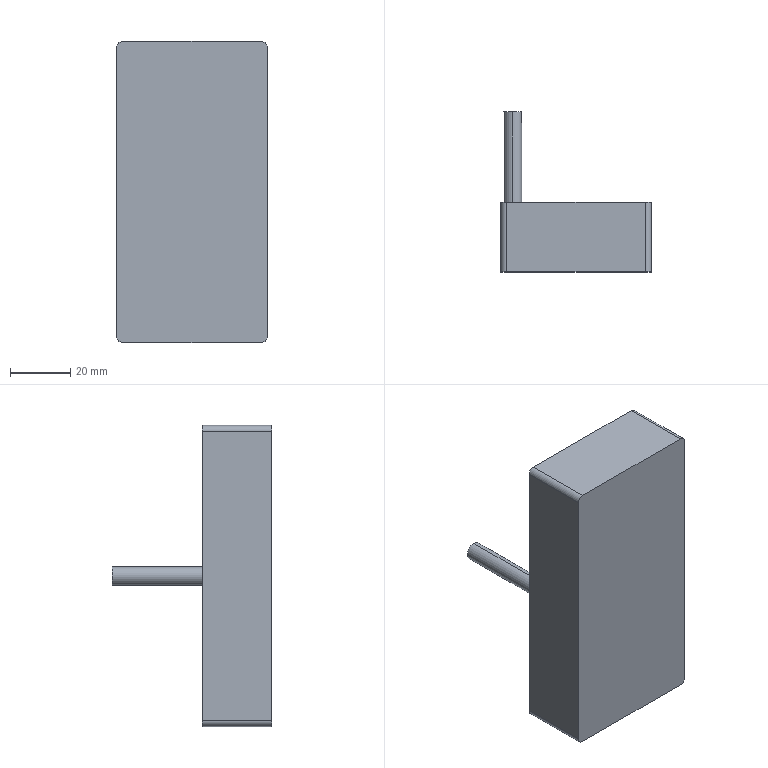Part | SolidWorks | features BaseBody 1 | 1 solid | 45 faces | box 50 x 53.1 x 100 mm | volume 115973 mm3 | cylinder 22 | cone 16 | plane 7 | commonest cylinder face diameters 3.3 x16 4 x4 6 x2
STEP:
#1=CARTESIAN_POINT('',(15.,19.1,86.85));
#2=VERTEX_POINT('',#1);
#3=CARTESIAN_POINT('',(15.,19.1,90.15));
#4=VERTEX_POINT('',#3);
#5=CARTESIAN_POINT('',(15.,19.1,88.5));
#6=DIRECTION('',(0.,1.,0.));
#7=DIRECTION('',(0.,0.,1.));
#8=AXIS2_PLACEMENT_3D('',#5,#6,#7);
#9=CIRCLE('',#8,1.65);
#10=EDGE_CURVE('',#2,#4,#9,.T.);
#11=ORIENTED_EDGE('',*,*,#10,.F.);
#12=CARTESIAN_POINT('',(15.,23.1,86.85));
#13=VERTEX_POINT('',#12);
#14=CARTESIAN_POINT('',(15.,23.1,86.85));
#15=DIRECTION('',(0.,1.,0.));
#16=VECTOR('',#15,1000.);
#17=LINE('',#14,#16);
#18=EDGE_CURVE('',#2,#13,#17,.T.);
#19=ORIENTED_EDGE('',*,*,#18,.T.);
#20=CARTESIAN_POINT('',(15.,23.1,90.15));
#21=VERTEX_POINT('',#20);
#22=CARTESIAN_POINT('',(15.,23.1,88.5));
#23=DIRECTION('',(0.,1.,0.));
#24=DIRECTION('',(0.,0.,1.));
#25=AXIS2_PLACEMENT_3D('',#22,#23,#24);
#26=CIRCLE('',#25,1.65);
#27=EDGE_CURVE('',#13,#21,#26,.T.);
#28=ORIENTED_EDGE('',*,*,#27,.T.);
#29=CARTESIAN_POINT('',(15.,23.1,90.15));
#30=DIRECTION('',(0.,1.,0.));
#31=VECTOR('',#30,1000.);
#32=LINE('',#29,#31);
#33=EDGE_CURVE('',#4,#21,#32,.T.);
#34=ORIENTED_EDGE('',*,*,#33,.F.);
#35=EDGE_LOOP('',(#11,#19,#28,#34));
#36=FACE_OUTER_BOUND('',#35,.T.);
#37=CARTESIAN_POINT('',(15.,23.1,88.5));
#38=DIRECTION('',(0.,1.,0.));
#39=DIRECTION('',(0.,0.,1.));
#40=AXIS2_PLACEMENT_3D('',#37,#38,#39);
#41=CYLINDRICAL_SURFACE('',#40,1.65);
#42=ADVANCED_FACE('',(#36),#41,.F.);
#43=CARTESIAN_POINT('',(15.,19.1,62.85));
#44=VERTEX_POINT('',#43);
#45=CARTESIAN_POINT('',(15.,19.1,66.15));
#46=VERTEX_POINT('',#45);
#47=CARTESIAN_POINT('',(15.,19.1,64.5));
#48=DIRECTION('',(0.,1.,0.));
#49=DIRECTION('',(0.,0.,1.));
#50=AXIS2_PLACEMENT_3D('',#47,#48,#49);
#51=CIRCLE('',#50,1.65);
#52=EDGE_CURVE('',#44,#46,#51,.T.);
#53=ORIENTED_EDGE('',*,*,#52,.F.);
#54=CARTESIAN_POINT('',(15.,23.1,62.85));
#55=VERTEX_POINT('',#54);
#56=CARTESIAN_POINT('',(15.,23.1,62.85));
#57=DIRECTION('',(0.,1.,0.));
#58=VECTOR('',#57,1000.);
#59=LINE('',#56,#58);
#60=EDGE_CURVE('',#44,#55,#59,.T.);
#61=ORIENTED_EDGE('',*,*,#60,.T.);
#62=CARTESIAN_POINT('',(15.,23.1,66.15));
#63=VERTEX_POINT('',#62);
#64=CARTESIAN_POINT('',(15.,23.1,64.5));
#65=DIRECTION('',(0.,1.,0.));
#66=DIRECTION('',(0.,0.,1.));
#67=AXIS2_PLACEMENT_3D('',#64,#65,#66);
#68=CIRCLE('',#67,1.65);
#69=EDGE_CURVE('',#55,#63,#68,.T.);
#70=ORIENTED_EDGE('',*,*,#69,.T.);
#71=CARTESIAN_POINT('',(15.,23.1,66.15));
#72=DIRECTION('',(0.,1.,0.));
#73=VECTOR('',#72,1000.);
#74=LINE('',#71,#73);
#75=EDGE_CURVE('',#46,#63,#74,.T.);
#76=ORIENTED_EDGE('',*,*,#75,.F.);
#77=EDGE_LOOP('',(#53,#61,#70,#76));
#78=FACE_OUTER_BOUND('',#77,.T.);
#79=CARTESIAN_POINT('',(15.,23.1,64.5));
#80=DIRECTION('',(0.,1.,0.));
#81=DIRECTION('',(0.,0.,1.));
#82=AXIS2_PLACEMENT_3D('',#79,#80,#81);
#83=CYLINDRICAL_SURFACE('',#82,1.65);
#84=ADVANCED_FACE('',(#78),#83,.F.);
#85=CARTESIAN_POINT('',(35.,19.1,86.85));
#86=VERTEX_POINT('',#85);
#87=CARTESIAN_POINT('',(35.,19.1,90.15));
#88=VERTEX_POINT('',#87);
#89=CARTESIAN_POINT('',(35.,19.1,88.5));
#90=DIRECTION('',(0.,1.,0.));
#91=DIRECTION('',(0.,0.,1.));
#92=AXIS2_PLACEMENT_3D('',#89,#90,#91);
#93=CIRCLE('',#92,1.65);
#94=EDGE_CURVE('',#86,#88,#93,.T.);
#95=ORIENTED_EDGE('',*,*,#94,.F.);
#96=CARTESIAN_POINT('',(35.,23.1,86.85));
#97=VERTEX_POINT('',#96);
#98=CARTESIAN_POINT('',(35.,23.1,86.85));
#99=DIRECTION('',(0.,1.,0.));
#100=VECTOR('',#99,1000.);
#101=LINE('',#98,#100);
#102=EDGE_CURVE('',#86,#97,#101,.T.);
#103=ORIENTED_EDGE('',*,*,#102,.T.);
#104=CARTESIAN_POINT('',(35.,23.1,90.15));
#105=VERTEX_POINT('',#104);
#106=CARTESIAN_POINT('',(35.,23.1,88.5));
#107=DIRECTION('',(0.,1.,0.));
#108=DIRECTION('',(0.,0.,1.));
#109=AXIS2_PLACEMENT_3D('',#106,#107,#108);
#110=CIRCLE('',#109,1.65);
#111=EDGE_CURVE('',#97,#105,#110,.T.);
#112=ORIENTED_EDGE('',*,*,#111,.T.);
#113=CARTESIAN_POINT('',(35.,23.1,90.15));
#114=DIRECTION('',(0.,1.,0.));
#115=VECTOR('',#114,1000.);
#116=LINE('',#113,#115);
#117=EDGE_CURVE('',#88,#105,#116,.T.);
#118=ORIENTED_EDGE('',*,*,#117,.F.);
#119=EDGE_LOOP('',(#95,#103,#112,#118));
#120=FACE_OUTER_BOUND('',#119,.T.);
#121=CARTESIAN_POINT('',(35.,23.1,88.5));
#122=DIRECTION('',(0.,1.,0.));
#123=DIRECTION('',(0.,0.,1.));
#124=AXIS2_PLACEMENT_3D('',#121,#122,#123);
#125=CYLINDRICAL_SURFACE('',#124,1.65);
#126=ADVANCED_FACE('',(#120),#125,.F.);
#127=CARTESIAN_POINT('',(35.,19.1,62.85));
#128=VERTEX_POINT('',#127);
#129=CARTESIAN_POINT('',(35.,19.1,66.15));
#130=VERTEX_POINT('',#129);
#131=CARTESIAN_POINT('',(35.,19.1,64.5));
#132=DIRECTION('',(0.,1.,0.));
#133=DIRECTION('',(0.,0.,1.));
#134=AXIS2_PLACEMENT_3D('',#131,#132,#133);
#135=CIRCLE('',#134,1.65);
#136=EDGE_CURVE('',#128,#130,#135,.T.);
#137=ORIENTED_EDGE('',*,*,#136,.F.);
#138=CARTESIAN_POINT('',(35.,23.1,62.85));
#139=VERTEX_POINT('',#138);
#140=CARTESIAN_POINT('',(35.,23.1,62.85));
#141=DIRECTION('',(0.,1.,0.));
#142=VECTOR('',#141,1000.);
#143=LINE('',#140,#142);
#144=EDGE_CURVE('',#128,#139,#143,.T.);
#145=ORIENTED_EDGE('',*,*,#144,.T.);
#146=CARTESIAN_POINT('',(35.,23.1,66.15));
#147=VERTEX_POINT('',#146);
#148=CARTESIAN_POINT('',(35.,23.1,64.5));
#149=DIRECTION('',(0.,1.,0.));
#150=DIRECTION('',(0.,0.,1.));
#151=AXIS2_PLACEMENT_3D('',#148,#149,#150);
#152=CIRCLE('',#151,1.65);
#153=EDGE_CURVE('',#139,#147,#152,.T.);
#154=ORIENTED_EDGE('',*,*,#153,.T.);
#155=CARTESIAN_POINT('',(35.,23.1,66.15));
#156=DIRECTION('',(0.,1.,0.));
#157=VECTOR('',#156,1000.);
#158=LINE('',#155,#157);
#159=EDGE_CURVE('',#130,#147,#158,.T.);
#160=ORIENTED_EDGE('',*,*,#159,.F.);
#161=EDGE_LOOP('',(#137,#145,#154,#160));
#162=FACE_OUTER_BOUND('',#161,.T.);
#163=CARTESIAN_POINT('',(35.,23.1,64.5));
#164=DIRECTION('',(0.,1.,0.));
#165=DIRECTION('',(0.,0.,1.));
#166=AXIS2_PLACEMENT_3D('',#163,#164,#165);
#167=CYLINDRICAL_SURFACE('',#166,1.65);
#168=ADVANCED_FACE('',(#162),#167,.F.);
#169=CARTESIAN_POINT('',(15.,19.1,14.85));
#170=VERTEX_POINT('',#169);
#171=CARTESIAN_POINT('',(15.,19.1,18.15));
#172=VERTEX_POINT('',#171);
#173=CARTESIAN_POINT('',(15.,19.1,16.5));
#174=DIRECTION('',(0.,1.,0.));
#175=DIRECTION('',(0.,0.,1.));
#176=AXIS2_PLACEMENT_3D('',#173,#174,#175);
#177=CIRCLE('',#176,1.65);
#178=EDGE_CURVE('',#170,#172,#177,.T.);
#179=ORIENTED_EDGE('',*,*,#178,.F.);
#180=CARTESIAN_POINT('',(15.,23.1,14.85));
#181=VERTEX_POINT('',#180);
#182=CARTESIAN_POINT('',(15.,23.1,14.85));
#183=DIRECTION('',(0.,1.,0.));
#184=VECTOR('',#183,1000.);
#185=LINE('',#182,#184);
#186=EDGE_CURVE('',#170,#181,#185,.T.);
#187=ORIENTED_EDGE('',*,*,#186,.T.);
#188=CARTESIAN_POINT('',(15.,23.1,18.15));
#189=VERTEX_POINT('',#188);
#190=CARTESIAN_POINT('',(15.,23.1,16.5));
#191=DIRECTION('',(0.,1.,0.));
#192=DIRECTION('',(0.,0.,1.));
#193=AXIS2_PLACEMENT_3D('',#190,#191,#192);
#194=CIRCLE('',#193,1.65);
#195=EDGE_CURVE('',#181,#189,#194,.T.);
#196=ORIENTED_EDGE('',*,*,#195,.T.);
#197=CARTESIAN_POINT('',(15.,23.1,18.15));
#198=DIRECTION('',(0.,1.,0.));
#199=VECTOR('',#198,1000.);
#200=LINE('',#197,#199);
#201=EDGE_CURVE('',#172,#189,#200,.T.);
#202=ORIENTED_EDGE('',*,*,#201,.F.);
#203=EDGE_LOOP('',(#179,#187,#196,#202));
#204=FACE_OUTER_BOUND('',#203,.T.);
#205=CARTESIAN_POINT('',(15.,23.1,16.5));
#206=DIRECTION('',(0.,1.,0.));
#207=DIRECTION('',(0.,0.,1.));
#208=AXIS2_PLACEMENT_3D('',#205,#206,#207);
#209=CYLINDRICAL_SURFACE('',#208,1.65);
#210=ADVANCED_FACE('',(#204),#209,.F.);
#211=CARTESIAN_POINT('',(35.,19.1,14.85));
#212=VERTEX_POINT('',#211);
#213=CARTESIAN_POINT('',(35.,19.1,18.15));
#214=VERTEX_POINT('',#213);
#215=CARTESIAN_POINT('',(35.,19.1,16.5));
#216=DIRECTION('',(0.,1.,0.));
#217=DIRECTION('',(0.,0.,1.));
#218=AXIS2_PLACEMENT_3D('',#215,#216,#217);
#219=CIRCLE('',#218,1.65);
#220=EDGE_CURVE('',#212,#214,#219,.T.);
#221=ORIENTED_EDGE('',*,*,#220,.F.);
#222=CARTESIAN_POINT('',(35.,23.1,14.85));
#223=VERTEX_POINT('',#222);
#224=CARTESIAN_POINT('',(35.,23.1,14.85));
#225=DIRECTION('',(0.,1.,0.));
#226=VECTOR('',#225,1000.);
#227=LINE('',#224,#226);
#228=EDGE_CURVE('',#212,#223,#227,.T.);
#229=ORIENTED_EDGE('',*,*,#228,.T.);
#230=CARTESIAN_POINT('',(35.,23.1,18.15));
#231=VERTEX_POINT('',#230);
#232=CARTESIAN_POINT('',(35.,23.1,16.5));
#233=DIRECTION('',(0.,1.,0.));
#234=DIRECTION('',(0.,0.,1.));
#235=AXIS2_PLACEMENT_3D('',#232,#233,#234);
#236=CIRCLE('',#235,1.65);
#237=EDGE_CURVE('',#223,#231,#236,.T.);
#238=ORIENTED_EDGE('',*,*,#237,.T.);
#239=CARTESIAN_POINT('',(35.,23.1,18.15));
#240=DIRECTION('',(0.,1.,0.));
#241=VECTOR('',#240,1000.);
#242=LINE('',#239,#241);
#243=EDGE_CURVE('',#214,#231,#242,.T.);
#244=ORIENTED_EDGE('',*,*,#243,.F.);
#245=EDGE_LOOP('',(#221,#229,#238,#244));
#246=FACE_OUTER_BOUND('',#245,.T.);
#247=CARTESIAN_POINT('',(35.,23.1,16.5));
#248=DIRECTION('',(0.,1.,0.));
#249=DIRECTION('',(0.,0.,1.));
#250=AXIS2_PLACEMENT_3D('',#247,#248,#249);
#251=CYLINDRICAL_SURFACE('',#250,1.65);
#252=ADVANCED_FACE('',(#246),#251,.F.);
#253=CARTESIAN_POINT('',(35.,19.1,38.85));
#254=VERTEX_POINT('',#253);
#255=CARTESIAN_POINT('',(35.,19.1,42.15));
#256=VERTEX_POINT('',#255);
#257=CARTESIAN_POINT('',(35.,19.1,40.5));
#258=DIRECTION('',(0.,1.,0.));
#259=DIRECTION('',(0.,0.,1.));
#260=AXIS2_PLACEMENT_3D('',#257,#258,#259);
#261=CIRCLE('',#260,1.65);
#262=EDGE_CURVE('',#254,#256,#261,.T.);
#263=ORIENTED_EDGE('',*,*,#262,.F.);
#264=CARTESIAN_POINT('',(35.,23.1,38.85));
#265=VERTEX_POINT('',#264);
#266=CARTESIAN_POINT('',(35.,23.1,38.85));
#267=DIRECTION('',(0.,1.,0.));
#268=VECTOR('',#267,1000.);
#269=LINE('',#266,#268);
#270=EDGE_CURVE('',#254,#265,#269,.T.);
#271=ORIENTED_EDGE('',*,*,#270,.T.);
#272=CARTESIAN_POINT('',(35.,23.1,42.15));
#273=VERTEX_POINT('',#272);
#274=CARTESIAN_POINT('',(35.,23.1,40.5));
#275=DIRECTION('',(0.,1.,0.));
#276=DIRECTION('',(0.,0.,1.));
#277=AXIS2_PLACEMENT_3D('',#274,#275,#276);
#278=CIRCLE('',#277,1.65);
#279=EDGE_CURVE('',#265,#273,#278,.T.);
#280=ORIENTED_EDGE('',*,*,#279,.T.);
#281=CARTESIAN_POINT('',(35.,23.1,42.15));
#282=DIRECTION('',(0.,1.,0.));
#283=VECTOR('',#282,1000.);
#284=LINE('',#281,#283);
#285=EDGE_CURVE('',#256,#273,#284,.T.);
#286=ORIENTED_EDGE('',*,*,#285,.F.);
#287=EDGE_LOOP('',(#263,#271,#280,#286));
#288=FACE_OUTER_BOUND('',#287,.T.);
#289=CARTESIAN_POINT('',(35.,23.1,40.5));
#290=DIRECTION('',(0.,1.,0.));
#291=DIRECTION('',(0.,0.,1.));
#292=AXIS2_PLACEMENT_3D('',#289,#290,#291);
#293=CYLINDRICAL_SURFACE('',#292,1.65);
#294=ADVANCED_FACE('',(#288),#293,.F.);
#295=CARTESIAN_POINT('',(15.,19.1,38.85));
#296=VERTEX_POINT('',#295);
#297=CARTESIAN_POINT('',(15.,19.1,42.15));
#298=VERTEX_POINT('',#297);
#299=CARTESIAN_POINT('',(15.,19.1,40.5));
#300=DIRECTION('',(0.,1.,0.));
#301=DIRECTION('',(0.,0.,1.));
#302=AXIS2_PLACEMENT_3D('',#299,#300,#301);
#303=CIRCLE('',#302,1.65);
#304=EDGE_CURVE('',#296,#298,#303,.T.);
#305=ORIENTED_EDGE('',*,*,#304,.F.);
#306=CARTESIAN_POINT('',(15.,23.1,38.85));
#307=VERTEX_POINT('',#306);
#308=CARTESIAN_POINT('',(15.,23.1,38.85));
#309=DIRECTION('',(0.,1.,0.));
#310=VECTOR('',#309,1000.);
#311=LINE('',#308,#310);
#312=EDGE_CURVE('',#296,#307,#311,.T.);
#313=ORIENTED_EDGE('',*,*,#312,.T.);
#314=CARTESIAN_POINT('',(15.,23.1,42.15));
#315=VERTEX_POINT('',#314);
#316=CARTESIAN_POINT('',(15.,23.1,40.5));
#317=DIRECTION('',(0.,1.,0.));
#318=DIRECTION('',(0.,0.,1.));
#319=AXIS2_PLACEMENT_3D('',#316,#317,#318);
#320=CIRCLE('',#319,1.65);
#321=EDGE_CURVE('',#307,#315,#320,.T.);
#322=ORIENTED_EDGE('',*,*,#321,.T.);
#323=CARTESIAN_POINT('',(15.,23.1,42.15));
#324=DIRECTION('',(0.,1.,0.));
#325=VECTOR('',#324,1000.);
#326=LINE('',#323,#325);
#327=EDGE_CURVE('',#298,#315,#326,.T.);
#328=ORIENTED_EDGE('',*,*,#327,.F.);
#329=EDGE_LOOP('',(#305,#313,#322,#328));
#330=FACE_OUTER_BOUND('',#329,.T.);
#331=CARTESIAN_POINT('',(15.,23.1,40.5));
#332=DIRECTION('',(0.,1.,0.));
#333=DIRECTION('',(0.,0.,1.));
#334=AXIS2_PLACEMENT_3D('',#331,#332,#333);
#335=CYLINDRICAL_SURFACE('',#334,1.65);
#336=ADVANCED_FACE('',(#330),#335,.F.);
#337=CARTESIAN_POINT('',(4.,53.1,47.));
#338=VERTEX_POINT('',#337);
#339=CARTESIAN_POINT('',(4.,53.1,53.));
#340=VERTEX_POINT('',#339);
#341=CARTESIAN_POINT('',(4.,53.1,50.));
#342=DIRECTION('',(0.,-1.,0.));
#343=DIRECTION('',(0.,0.,-1.));
#344=AXIS2_PLACEMENT_3D('',#341,#342,#343);
#345=CIRCLE('',#344,3.);
#346=EDGE_CURVE('',#338,#340,#345,.T.);
#347=ORIENTED_EDGE('',*,*,#346,.T.);
#348=CARTESIAN_POINT('',(4.,23.1,53.));
#349=VERTEX_POINT('',#348);
#350=CARTESIAN_POINT('',(4.,53.1,53.));
#351=DIRECTION('',(0.,-1.,0.));
#352=VECTOR('',#351,1000.);
#353=LINE('',#350,#352);
#354=EDGE_CURVE('',#340,#349,#353,.T.);
#355=ORIENTED_EDGE('',*,*,#354,.T.);
#356=CARTESIAN_POINT('',(4.,23.1,47.));
#357=VERTEX_POINT('',#356);
#358=CARTESIAN_POINT('',(4.,23.1,50.));
#359=DIRECTION('',(0.,1.,0.));
#360=DIRECTION('',(0.,0.,-1.));
#361=AXIS2_PLACEMENT_3D('',#358,#359,#360);
#362=CIRCLE('',#361,3.);
#363=EDGE_CURVE('',#349,#357,#362,.T.);
#364=ORIENTED_EDGE('',*,*,#363,.T.);
#365=CARTESIAN_POINT('',(4.,53.1,47.));
#366=DIRECTION('',(0.,-1.,0.));
#367=VECTOR('',#366,1000.);
#368=LINE('',#365,#367);
#369=EDGE_CURVE('',#338,#357,#368,.T.);
#370=ORIENTED_EDGE('',*,*,#369,.F.);
#371=EDGE_LOOP('',(#347,#355,#364,#370));
#372=FACE_OUTER_BOUND('',#371,.T.);
#373=CARTESIAN_POINT('',(4.,53.1,50.));
#374=DIRECTION('',(0.,-1.,0.));
#375=DIRECTION('',(0.,0.,-1.));
#376=AXIS2_PLACEMENT_3D('',#373,#374,#375);
#377=CYLINDRICAL_SURFACE('',#376,3.);
#378=ADVANCED_FACE('',(#372),#377,.T.);
#379=CARTESIAN_POINT('',(15.,18.109,88.5));
#380=VERTEX_POINT('',#379);
#381=CARTESIAN_POINT('',(15.,19.1,90.15));
#382=DIRECTION('',(0.,0.515,0.8572));
#383=VECTOR('',#382,1000.);
#384=LINE('',#381,#383);
#385=EDGE_CURVE('',#380,#4,#384,.T.);
#386=ORIENTED_EDGE('',*,*,#385,.F.);
#387=CARTESIAN_POINT('',(15.,19.1,86.85));
#388=DIRECTION('',(0.,0.515,-0.8572));
#389=VECTOR('',#388,1000.);
#390=LINE('',#387,#389);
#391=EDGE_CURVE('',#380,#2,#390,.T.);
#392=ORIENTED_EDGE('',*,*,#391,.T.);
#393=ORIENTED_EDGE('',*,*,#10,.T.);
#394=EDGE_LOOP('',(#386,#392,#393));
#395=FACE_OUTER_BOUND('',#394,.T.);
#396=CARTESIAN_POINT('',(15.,19.1,88.5));
#397=DIRECTION('',(0.,1.,0.));
#398=DIRECTION('',(0.,0.,1.));
#399=AXIS2_PLACEMENT_3D('',#396,#397,#398);
#400=CONICAL_SURFACE('',#399,1.65,1.03);
#401=ADVANCED_FACE('',(#395),#400,.F.);
#402=CARTESIAN_POINT('',(15.,18.109,64.5));
#403=VERTEX_POINT('',#402);
#404=CARTESIAN_POINT('',(15.,19.1,66.15));
#405=DIRECTION('',(0.,0.515,0.8572));
#406=VECTOR('',#405,1000.);
#407=LINE('',#404,#406);
#408=EDGE_CURVE('',#403,#46,#407,.T.);
#409=ORIENTED_EDGE('',*,*,#408,.F.);
#410=CARTESIAN_POINT('',(15.,19.1,62.85));
#411=DIRECTION('',(0.,0.515,-0.8572));
#412=VECTOR('',#411,1000.);
#413=LINE('',#410,#412);
#414=EDGE_CURVE('',#403,#44,#413,.T.);
#415=ORIENTED_EDGE('',*,*,#414,.T.);
#416=ORIENTED_EDGE('',*,*,#52,.T.);
#417=EDGE_LOOP('',(#409,#415,#416));
#418=FACE_OUTER_BOUND('',#417,.T.);
#419=CARTESIAN_POINT('',(15.,19.1,64.5));
#420=DIRECTION('',(0.,1.,0.));
#421=DIRECTION('',(0.,0.,1.));
#422=AXIS2_PLACEMENT_3D('',#419,#420,#421);
#423=CONICAL_SURFACE('',#422,1.65,1.03);
#424=ADVANCED_FACE('',(#418),#423,.F.);
#425=CARTESIAN_POINT('',(35.,18.109,88.5));
#426=VERTEX_POINT('',#425);
#427=CARTESIAN_POINT('',(35.,19.1,90.15));
#428=DIRECTION('',(0.,0.515,0.8572));
#429=VECTOR('',#428,1000.);
#430=LINE('',#427,#429);
#431=EDGE_CURVE('',#426,#88,#430,.T.);
#432=ORIENTED_EDGE('',*,*,#431,.F.);
#433=CARTESIAN_POINT('',(35.,19.1,86.85));
#434=DIRECTION('',(0.,0.515,-0.8572));
#435=VECTOR('',#434,1000.);
#436=LINE('',#433,#435);
#437=EDGE_CURVE('',#426,#86,#436,.T.);
#438=ORIENTED_EDGE('',*,*,#437,.T.);
#439=ORIENTED_EDGE('',*,*,#94,.T.);
#440=EDGE_LOOP('',(#432,#438,#439));
#441=FACE_OUTER_BOUND('',#440,.T.);
#442=CARTESIAN_POINT('',(35.,19.1,88.5));
#443=DIRECTION('',(0.,1.,0.));
#444=DIRECTION('',(0.,0.,1.));
#445=AXIS2_PLACEMENT_3D('',#442,#443,#444);
#446=CONICAL_SURFACE('',#445,1.65,1.03);
#447=ADVANCED_FACE('',(#441),#446,.F.);
#448=CARTESIAN_POINT('',(35.,18.109,64.5));
#449=VERTEX_POINT('',#448);
#450=CARTESIAN_POINT('',(35.,19.1,66.15));
#451=DIRECTION('',(0.,0.515,0.8572));
#452=VECTOR('',#451,1000.);
#453=LINE('',#450,#452);
#454=EDGE_CURVE('',#449,#130,#453,.T.);
#455=ORIENTED_EDGE('',*,*,#454,.F.);
#456=CARTESIAN_POINT('',(35.,19.1,62.85));
#457=DIRECTION('',(0.,0.515,-0.8572));
#458=VECTOR('',#457,1000.);
#459=LINE('',#456,#458);
#460=EDGE_CURVE('',#449,#128,#459,.T.);
#461=ORIENTED_EDGE('',*,*,#460,.T.);
#462=ORIENTED_EDGE('',*,*,#136,.T.);
#463=EDGE_LOOP('',(#455,#461,#462));
#464=FACE_OUTER_BOUND('',#463,.T.);
#465=CARTESIAN_POINT('',(35.,19.1,64.5));
#466=DIRECTION('',(0.,1.,0.));
#467=DIRECTION('',(0.,0.,1.));
#468=AXIS2_PLACEMENT_3D('',#465,#466,#467);
#469=CONICAL_SURFACE('',#468,1.65,1.03);
#470=ADVANCED_FACE('',(#464),#469,.F.);
#471=CARTESIAN_POINT('',(15.,18.109,16.5));
#472=VERTEX_POINT('',#471);
#473=CARTESIAN_POINT('',(15.,19.1,18.15));
#474=DIRECTION('',(0.,0.515,0.8572));
#475=VECTOR('',#474,1000.);
#476=LINE('',#473,#475);
#477=EDGE_CURVE('',#472,#172,#476,.T.);
#478=ORIENTED_EDGE('',*,*,#477,.F.);
#479=CARTESIAN_POINT('',(15.,19.1,14.85));
#480=DIRECTION('',(0.,0.515,-0.8572));
#481=VECTOR('',#480,1000.);
#482=LINE('',#479,#481);
#483=EDGE_CURVE('',#472,#170,#482,.T.);
#484=ORIENTED_EDGE('',*,*,#483,.T.);
#485=ORIENTED_EDGE('',*,*,#178,.T.);
#486=EDGE_LOOP('',(#478,#484,#485));
#487=FACE_OUTER_BOUND('',#486,.T.);
#488=CARTESIAN_POINT('',(15.,19.1,16.5));
#489=DIRECTION('',(0.,1.,0.));
#490=DIRECTION('',(0.,0.,1.));
#491=AXIS2_PLACEMENT_3D('',#488,#489,#490);
#492=CONICAL_SURFACE('',#491,1.65,1.03);
#493=ADVANCED_FACE('',(#487),#492,.F.);
#494=CARTESIAN_POINT('',(35.,18.109,16.5));
#495=VERTEX_POINT('',#494);
#496=CARTESIAN_POINT('',(35.,19.1,18.15));
#497=DIRECTION('',(0.,0.515,0.8572));
#498=VECTOR('',#497,1000.);
#499=LINE('',#496,#498);
#500=EDGE_CURVE('',#495,#214,#499,.T.);
#501=ORIENTED_EDGE('',*,*,#500,.F.);
#502=CARTESIAN_POINT('',(35.,19.1,14.85));
#503=DIRECTION('',(0.,0.515,-0.8572));
#504=VECTOR('',#503,1000.);
#505=LINE('',#502,#504);
#506=EDGE_CURVE('',#495,#212,#505,.T.);
#507=ORIENTED_EDGE('',*,*,#506,.T.);
#508=ORIENTED_EDGE('',*,*,#220,.T.);
#509=EDGE_LOOP('',(#501,#507,#508));
#510=FACE_OUTER_BOUND('',#509,.T.);
#511=CARTESIAN_POINT('',(35.,19.1,16.5));
#512=DIRECTION('',(0.,1.,0.));
#513=DIRECTION('',(0.,0.,1.));
#514=AXIS2_PLACEMENT_3D('',#511,#512,#513);
#515=CONICAL_SURFACE('',#514,1.65,1.03);
#516=ADVANCED_FACE('',(#510),#515,.F.);
#517=CARTESIAN_POINT('',(35.,18.109,40.5));
#518=VERTEX_POINT('',#517);
#519=CARTESIAN_POINT('',(35.,19.1,42.15));
#520=DIRECTION('',(0.,0.515,0.8572));
#521=VECTOR('',#520,1000.);
#522=LINE('',#519,#521);
#523=EDGE_CURVE('',#518,#256,#522,.T.);
#524=ORIENTED_EDGE('',*,*,#523,.F.);
#525=CARTESIAN_POINT('',(35.,19.1,38.85));
#526=DIRECTION('',(0.,0.515,-0.8572));
#527=VECTOR('',#526,1000.);
#528=LINE('',#525,#527);
#529=EDGE_CURVE('',#518,#254,#528,.T.);
#530=ORIENTED_EDGE('',*,*,#529,.T.);
#531=ORIENTED_EDGE('',*,*,#262,.T.);
#532=EDGE_LOOP('',(#524,#530,#531));
#533=FACE_OUTER_BOUND('',#532,.T.);
#534=CARTESIAN_POINT('',(35.,19.1,40.5));
#535=DIRECTION('',(0.,1.,0.));
#536=DIRECTION('',(0.,0.,1.));
#537=AXIS2_PLACEMENT_3D('',#534,#535,#536);
#538=CONICAL_SURFACE('',#537,1.65,1.03);
#539=ADVANCED_FACE('',(#533),#538,.F.);
#540=CARTESIAN_POINT('',(15.,18.109,40.5));
#541=VERTEX_POINT('',#540);
#542=CARTESIAN_POINT('',(15.,19.1,42.15));
#543=DIRECTION('',(0.,0.515,0.8572));
#544=VECTOR('',#543,1000.);
#545=LINE('',#542,#544);
#546=EDGE_CURVE('',#541,#298,#545,.T.);
#547=ORIENTED_EDGE('',*,*,#546,.F.);
#548=CARTESIAN_POINT('',(15.,19.1,38.85));
#549=DIRECTION('',(0.,0.515,-0.8572));
#550=VECTOR('',#549,1000.);
#551=LINE('',#548,#550);
#552=EDGE_CURVE('',#541,#296,#551,.T.);
#553=ORIENTED_EDGE('',*,*,#552,.T.);
#554=ORIENTED_EDGE('',*,*,#304,.T.);
#555=EDGE_LOOP('',(#547,#553,#554));
#556=FACE_OUTER_BOUND('',#555,.T.);
#557=CARTESIAN_POINT('',(15.,19.1,40.5));
#558=DIRECTION('',(0.,1.,0.));
#559=DIRECTION('',(0.,0.,1.));
#560=AXIS2_PLACEMENT_3D('',#557,#558,#559);
#561=CONICAL_SURFACE('',#560,1.65,1.03);
#562=ADVANCED_FACE('',(#556),#561,.F.);
#563=CARTESIAN_POINT('',(2.,0.,0.));
#564=VERTEX_POINT('',#563);
#565=CARTESIAN_POINT('',(0.,0.,2.));
#566=VERTEX_POINT('',#565);
#567=CARTESIAN_POINT('',(2.,0.,2.));
#568=DIRECTION('',(0.,1.,0.));
#569=DIRECTION('',(0.,0.,1.));
#570=AXIS2_PLACEMENT_3D('',#567,#568,#569);
#571=CIRCLE('',#570,2.);
#572=EDGE_CURVE('',#564,#566,#571,.T.);
#573=ORIENTED_EDGE('',*,*,#572,.F.);
#574=CARTESIAN_POINT('',(48.,0.,0.));
#575=VERTEX_POINT('',#574);
#576=CARTESIAN_POINT('',(0.,0.,0.));
#577=DIRECTION('',(-1.,0.,0.));
#578=VECTOR('',#577,1000.);
#579=LINE('',#576,#578);
#580=EDGE_CURVE('',#575,#564,#579,.T.);
#581=ORIENTED_EDGE('',*,*,#580,.F.);
#582=CARTESIAN_POINT('',(50.,0.,2.));
#583=VERTEX_POINT('',#582);
#584=CARTESIAN_POINT('',(48.,0.,2.));
#585=DIRECTION('',(0.,1.,0.));
#586=DIRECTION('',(0.,0.,-1.));
#587=AXIS2_PLACEMENT_3D('',#584,#585,#586);
#588=CIRCLE('',#587,2.);
#589=EDGE_CURVE('',#583,#575,#588,.T.);
#590=ORIENTED_EDGE('',*,*,#589,.F.);
#591=CARTESIAN_POINT('',(50.,0.,98.));
#592=VERTEX_POINT('',#591);
#593=CARTESIAN_POINT('',(50.,0.,100.));
#594=DIRECTION('',(0.,0.,-1.));
#595=VECTOR('',#594,1000.);
#596=LINE('',#593,#595);
#597=EDGE_CURVE('',#592,#583,#596,.T.);
#598=ORIENTED_EDGE('',*,*,#597,.F.);
#599=CARTESIAN_POINT('',(48.,0.,100.));
#600=VERTEX_POINT('',#599);
#601=CARTESIAN_POINT('',(48.,0.,98.));
#602=DIRECTION('',(0.,1.,0.));
#603=DIRECTION('',(0.,0.,1.));
#604=AXIS2_PLACEMENT_3D('',#601,#602,#603);
#605=CIRCLE('',#604,2.);
#606=EDGE_CURVE('',#600,#592,#605,.T.);
#607=ORIENTED_EDGE('',*,*,#606,.F.);
#608=CARTESIAN_POINT('',(2.,0.,100.));
#609=VERTEX_POINT('',#608);
#610=CARTESIAN_POINT('',(0.,0.,100.));
#611=DIRECTION('',(1.,0.,0.));
#612=VECTOR('',#611,1000.);
#613=LINE('',#610,#612);
#614=EDGE_CURVE('',#609,#600,#613,.T.);
#615=ORIENTED_EDGE('',*,*,#614,.F.);
#616=CARTESIAN_POINT('',(0.,0.,98.));
#617=VERTEX_POINT('',#616);
#618=CARTESIAN_POINT('',(2.,0.,98.));
#619=DIRECTION('',(0.,1.,0.));
#620=DIRECTION('',(0.,0.,-1.));
#621=AXIS2_PLACEMENT_3D('',#618,#619,#620);
#622=CIRCLE('',#621,2.);
#623=EDGE_CURVE('',#617,#609,#622,.T.);
#624=ORIENTED_EDGE('',*,*,#623,.F.);
#625=CARTESIAN_POINT('',(0.,0.,100.));
#626=DIRECTION('',(0.,0.,1.));
#627=VECTOR('',#626,1000.);
#628=LINE('',#625,#627);
#629=EDGE_CURVE('',#566,#617,#628,.T.);
#630=ORIENTED_EDGE('',*,*,#629,.F.);
#631=EDGE_LOOP('',(#573,#581,#590,#598,#607,#615,#624,#630));
#632=FACE_OUTER_BOUND('',#631,.T.);
#633=CARTESIAN_POINT('',(0.,0.,100.));
#634=DIRECTION('',(0.,1.,0.));
#635=DIRECTION('',(0.,0.,1.));
#636=AXIS2_PLACEMENT_3D('',#633,#634,#635);
#637=PLANE('',#636);
#638=ADVANCED_FACE('',(#632),#637,.F.);
#639=CARTESIAN_POINT('',(0.,23.1,2.));
#640=VERTEX_POINT('',#639);
#641=CARTESIAN_POINT('',(0.,0.,2.));
#642=DIRECTION('',(0.,1.,0.));
#643=VECTOR('',#642,1000.);
#644=LINE('',#641,#643);
#645=EDGE_CURVE('',#566,#640,#644,.T.);
#646=ORIENTED_EDGE('',*,*,#645,.F.);
#647=ORIENTED_EDGE('',*,*,#629,.T.);
#648=CARTESIAN_POINT('',(0.,23.1,98.));
#649=VERTEX_POINT('',#648);
#650=CARTESIAN_POINT('',(0.,0.,98.));
#651=DIRECTION('',(0.,-1.,0.));
#652=VECTOR('',#651,1000.);
#653=LINE('',#650,#652);
#654=EDGE_CURVE('',#649,#617,#653,.T.);
#655=ORIENTED_EDGE('',*,*,#654,.F.);
#656=CARTESIAN_POINT('',(0.,23.1,100.));
#657=DIRECTION('',(0.,0.,1.));
#658=VECTOR('',#657,1000.);
#659=LINE('',#656,#658);
#660=EDGE_CURVE('',#640,#649,#659,.T.);
#661=ORIENTED_EDGE('',*,*,#660,.F.);
#662=EDGE_LOOP('',(#646,#647,#655,#661));
#663=FACE_OUTER_BOUND('',#662,.T.);
#664=CARTESIAN_POINT('',(0.,0.,100.));
#665=DIRECTION('',(1.,0.,0.));
#666=DIRECTION('',(0.,0.,-1.));
#667=AXIS2_PLACEMENT_3D('',#664,#665,#666);
#668=PLANE('',#667);
#669=ADVANCED_FACE('',(#663),#668,.F.);
#670=ORIENTED_EDGE('',*,*,#572,.T.);
#671=ORIENTED_EDGE('',*,*,#645,.T.);
#672=CARTESIAN_POINT('',(2.,23.1,0.));
#673=VERTEX_POINT('',#672);
#674=CARTESIAN_POINT('',(2.,23.1,2.));
#675=DIRECTION('',(0.,-1.,0.));
#676=DIRECTION('',(0.,0.,1.));
#677=AXIS2_PLACEMENT_3D('',#674,#675,#676);
#678=CIRCLE('',#677,2.);
#679=EDGE_CURVE('',#640,#673,#678,.T.);
#680=ORIENTED_EDGE('',*,*,#679,.T.);
#681=CARTESIAN_POINT('',(2.,0.,0.));
#682=DIRECTION('',(0.,-1.,0.));
#683=VECTOR('',#682,1000.);
#684=LINE('',#681,#683);
#685=EDGE_CURVE('',#673,#564,#684,.T.);
#686=ORIENTED_EDGE('',*,*,#685,.T.);
#687=EDGE_LOOP('',(#670,#671,#680,#686));
#688=FACE_OUTER_BOUND('',#687,.T.);
#689=CARTESIAN_POINT('',(2.,0.,2.));
#690=DIRECTION('',(0.,1.,0.));
#691=DIRECTION('',(0.,0.,1.));
#692=AXIS2_PLACEMENT_3D('',#689,#690,#691);
#693=CYLINDRICAL_SURFACE('',#692,2.);
#694=ADVANCED_FACE('',(#688),#693,.T.);
#695=CARTESIAN_POINT('',(48.,23.1,0.));
#696=VERTEX_POINT('',#695);
#697=CARTESIAN_POINT('',(0.,23.1,0.));
#698=DIRECTION('',(1.,0.,0.));
#699=VECTOR('',#698,1000.);
#700=LINE('',#697,#699);
#701=EDGE_CURVE('',#673,#696,#700,.T.);
#702=ORIENTED_EDGE('',*,*,#701,.T.);
#703=CARTESIAN_POINT('',(48.,0.,0.));
#704=DIRECTION('',(0.,-1.,0.));
#705=VECTOR('',#704,1000.);
#706=LINE('',#703,#705);
#707=EDGE_CURVE('',#696,#575,#706,.T.);
#708=ORIENTED_EDGE('',*,*,#707,.T.);
#709=ORIENTED_EDGE('',*,*,#580,.T.);
#710=ORIENTED_EDGE('',*,*,#685,.F.);
#711=EDGE_LOOP('',(#702,#708,#709,#710));
#712=FACE_OUTER_BOUND('',#711,.T.);
#713=CARTESIAN_POINT('',(0.,0.,0.));
#714=DIRECTION('',(0.,0.,-1.));
#715=DIRECTION('',(-1.,0.,0.));
#716=AXIS2_PLACEMENT_3D('',#713,#714,#715);
#717=PLANE('',#716);
#718=ADVANCED_FACE('',(#712),#717,.T.);
#719=CARTESIAN_POINT('',(50.,23.1,2.));
#720=VERTEX_POINT('',#719);
#721=CARTESIAN_POINT('',(48.,23.1,2.));
#722=DIRECTION('',(0.,-1.,0.));
#723=DIRECTION('',(0.,0.,-1.));
#724=AXIS2_PLACEMENT_3D('',#721,#722,#723);
#725=CIRCLE('',#724,2.);
#726=EDGE_CURVE('',#696,#720,#725,.T.);
#727=ORIENTED_EDGE('',*,*,#726,.T.);
#728=CARTESIAN_POINT('',(50.,0.,2.));
#729=DIRECTION('',(0.,-1.,0.));
#730=VECTOR('',#729,1000.);
#731=LINE('',#728,#730);
#732=EDGE_CURVE('',#720,#583,#731,.T.);
#733=ORIENTED_EDGE('',*,*,#732,.T.);
#734=ORIENTED_EDGE('',*,*,#589,.T.);
#735=ORIENTED_EDGE('',*,*,#707,.F.);
#736=EDGE_LOOP('',(#727,#733,#734,#735));
#737=FACE_OUTER_BOUND('',#736,.T.);
#738=CARTESIAN_POINT('',(48.,0.,2.));
#739=DIRECTION('',(0.,-1.,0.));
#740=DIRECTION('',(0.,0.,-1.));
#741=AXIS2_PLACEMENT_3D('',#738,#739,#740);
#742=CYLINDRICAL_SURFACE('',#741,2.);
#743=ADVANCED_FACE('',(#737),#742,.T.);
#744=ORIENTED_EDGE('',*,*,#732,.F.);
#745=CARTESIAN_POINT('',(50.,23.1,98.));
#746=VERTEX_POINT('',#745);
#747=CARTESIAN_POINT('',(50.,23.1,100.));
#748=DIRECTION('',(0.,0.,-1.));
#749=VECTOR('',#748,1000.);
#750=LINE('',#747,#749);
#751=EDGE_CURVE('',#746,#720,#750,.T.);
#752=ORIENTED_EDGE('',*,*,#751,.F.);
#753=CARTESIAN_POINT('',(50.,0.,98.));
#754=DIRECTION('',(0.,1.,0.));
#755=VECTOR('',#754,1000.);
#756=LINE('',#753,#755);
#757=EDGE_CURVE('',#592,#746,#756,.T.);
#758=ORIENTED_EDGE('',*,*,#757,.F.);
#759=ORIENTED_EDGE('',*,*,#597,.T.);
#760=EDGE_LOOP('',(#744,#752,#758,#759));
#761=FACE_OUTER_BOUND('',#760,.T.);
#762=CARTESIAN_POINT('',(50.,0.,100.));
#763=DIRECTION('',(-1.,0.,0.));
#764=DIRECTION('',(0.,0.,1.));
#765=AXIS2_PLACEMENT_3D('',#762,#763,#764);
#766=PLANE('',#765);
#767=ADVANCED_FACE('',(#761),#766,.F.);
#768=CARTESIAN_POINT('',(48.,23.1,100.));
#769=VERTEX_POINT('',#768);
#770=CARTESIAN_POINT('',(48.,23.1,98.));
#771=DIRECTION('',(0.,-1.,0.));
#772=DIRECTION('',(0.,0.,1.));
#773=AXIS2_PLACEMENT_3D('',#770,#771,#772);
#774=CIRCLE('',#773,2.);
#775=EDGE_CURVE('',#746,#769,#774,.T.);
#776=ORIENTED_EDGE('',*,*,#775,.T.);
#777=CARTESIAN_POINT('',(48.,0.,100.));
#778=DIRECTION('',(0.,-1.,0.));
#779=VECTOR('',#778,1000.);
#780=LINE('',#777,#779);
#781=EDGE_CURVE('',#769,#600,#780,.T.);
#782=ORIENTED_EDGE('',*,*,#781,.T.);
#783=ORIENTED_EDGE('',*,*,#606,.T.);
#784=ORIENTED_EDGE('',*,*,#757,.T.);
#785=EDGE_LOOP('',(#776,#782,#783,#784));
#786=FACE_OUTER_BOUND('',#785,.T.);
#787=CARTESIAN_POINT('',(48.,0.,98.));
#788=DIRECTION('',(0.,1.,0.));
#789=DIRECTION('',(0.,0.,1.));
#790=AXIS2_PLACEMENT_3D('',#787,#788,#789);
#791=CYLINDRICAL_SURFACE('',#790,2.);
#792=ADVANCED_FACE('',(#786),#791,.T.);
#793=ORIENTED_EDGE('',*,*,#781,.F.);
#794=CARTESIAN_POINT('',(2.,23.1,100.));
#795=VERTEX_POINT('',#794);
#796=CARTESIAN_POINT('',(0.,23.1,100.));
#797=DIRECTION('',(1.,0.,0.));
#798=VECTOR('',#797,1000.);
#799=LINE('',#796,#798);
#800=EDGE_CURVE('',#795,#769,#799,.T.);
#801=ORIENTED_EDGE('',*,*,#800,.F.);
#802=CARTESIAN_POINT('',(2.,0.,100.));
#803=DIRECTION('',(0.,1.,0.));
#804=VECTOR('',#803,1000.);
#805=LINE('',#802,#804);
#806=EDGE_CURVE('',#609,#795,#805,.T.);
#807=ORIENTED_EDGE('',*,*,#806,.F.);
#808=ORIENTED_EDGE('',*,*,#614,.T.);
#809=EDGE_LOOP('',(#793,#801,#807,#808));
#810=FACE_OUTER_BOUND('',#809,.T.);
#811=CARTESIAN_POINT('',(0.,0.,100.));
#812=DIRECTION('',(0.,0.,-1.));
#813=DIRECTION('',(-1.,0.,0.));
#814=AXIS2_PLACEMENT_3D('',#811,#812,#813);
#815=PLANE('',#814);
#816=ADVANCED_FACE('',(#810),#815,.F.);
#817=ORIENTED_EDGE('',*,*,#623,.T.);
#818=ORIENTED_EDGE('',*,*,#806,.T.);
#819=CARTESIAN_POINT('',(2.,23.1,98.));
#820=DIRECTION('',(0.,-1.,0.));
#821=DIRECTION('',(0.,0.,-1.));
#822=AXIS2_PLACEMENT_3D('',#819,#820,#821);
#823=CIRCLE('',#822,2.);
#824=EDGE_CURVE('',#795,#649,#823,.T.);
#825=ORIENTED_EDGE('',*,*,#824,.T.);
#826=ORIENTED_EDGE('',*,*,#654,.T.);
#827=EDGE_LOOP('',(#817,#818,#825,#826));
#828=FACE_OUTER_BOUND('',#827,.T.);
#829=CARTESIAN_POINT('',(2.,0.,98.));
#830=DIRECTION('',(0.,-1.,0.));
#831=DIRECTION('',(0.,0.,-1.));
#832=AXIS2_PLACEMENT_3D('',#829,#830,#831);
#833=CYLINDRICAL_SURFACE('',#832,2.);
#834=ADVANCED_FACE('',(#828),#833,.T.);
#835=CARTESIAN_POINT('',(15.,23.1,88.5));
#836=DIRECTION('',(0.,1.,0.));
#837=DIRECTION('',(0.,0.,1.));
#838=AXIS2_PLACEMENT_3D('',#835,#836,#837);
#839=CIRCLE('',#838,1.65);
#840=EDGE_CURVE('',#21,#13,#839,.T.);
#841=ORIENTED_EDGE('',*,*,#840,.F.);
#842=ORIENTED_EDGE('',*,*,#27,.F.);
#843=EDGE_LOOP('',(#841,#842));
#844=FACE_BOUND('',#843,.T.);
#845=CARTESIAN_POINT('',(15.,23.1,64.5));
#846=DIRECTION('',(0.,1.,0.));
#847=DIRECTION('',(0.,0.,1.));
#848=AXIS2_PLACEMENT_3D('',#845,#846,#847);
#849=CIRCLE('',#848,1.65);
#850=EDGE_CURVE('',#63,#55,#849,.T.);
#851=ORIENTED_EDGE('',*,*,#850,.F.);
#852=ORIENTED_EDGE('',*,*,#69,.F.);
#853=EDGE_LOOP('',(#851,#852));
#854=FACE_BOUND('',#853,.T.);
#855=CARTESIAN_POINT('',(35.,23.1,88.5));
#856=DIRECTION('',(0.,1.,0.));
#857=DIRECTION('',(0.,0.,1.));
#858=AXIS2_PLACEMENT_3D('',#855,#856,#857);
#859=CIRCLE('',#858,1.65);
#860=EDGE_CURVE('',#105,#97,#859,.T.);
#861=ORIENTED_EDGE('',*,*,#860,.F.);
#862=ORIENTED_EDGE('',*,*,#111,.F.);
#863=EDGE_LOOP('',(#861,#862));
#864=FACE_BOUND('',#863,.T.);
#865=CARTESIAN_POINT('',(35.,23.1,64.5));
#866=DIRECTION('',(0.,1.,0.));
#867=DIRECTION('',(0.,0.,1.));
#868=AXIS2_PLACEMENT_3D('',#865,#866,#867);
#869=CIRCLE('',#868,1.65);
#870=EDGE_CURVE('',#147,#139,#869,.T.);
#871=ORIENTED_EDGE('',*,*,#870,.F.);
#872=ORIENTED_EDGE('',*,*,#153,.F.);
#873=EDGE_LOOP('',(#871,#872));
#874=FACE_BOUND('',#873,.T.);
#875=ORIENTED_EDGE('',*,*,#679,.F.);
#876=ORIENTED_EDGE('',*,*,#660,.T.);
#877=ORIENTED_EDGE('',*,*,#824,.F.);
#878=ORIENTED_EDGE('',*,*,#800,.T.);
#879=ORIENTED_EDGE('',*,*,#775,.F.);
#880=ORIENTED_EDGE('',*,*,#751,.T.);
#881=ORIENTED_EDGE('',*,*,#726,.F.);
#882=ORIENTED_EDGE('',*,*,#701,.F.);
#883=EDGE_LOOP('',(#875,#876,#877,#878,#879,#880,#881,#882));
#884=FACE_OUTER_BOUND('',#883,.T.);
#885=CARTESIAN_POINT('',(15.,23.1,16.5));
#886=DIRECTION('',(0.,1.,0.));
#887=DIRECTION('',(0.,0.,1.));
#888=AXIS2_PLACEMENT_3D('',#885,#886,#887);
#889=CIRCLE('',#888,1.65);
#890=EDGE_CURVE('',#189,#181,#889,.T.);
#891=ORIENTED_EDGE('',*,*,#890,.F.);
#892=ORIENTED_EDGE('',*,*,#195,.F.);
#893=EDGE_LOOP('',(#891,#892));
#894=FACE_BOUND('',#893,.T.);
#895=CARTESIAN_POINT('',(35.,23.1,16.5));
#896=DIRECTION('',(0.,1.,0.));
#897=DIRECTION('',(0.,0.,1.));
#898=AXIS2_PLACEMENT_3D('',#895,#896,#897);
#899=CIRCLE('',#898,1.65);
#900=EDGE_CURVE('',#231,#223,#899,.T.);
#901=ORIENTED_EDGE('',*,*,#900,.F.);
#902=ORIENTED_EDGE('',*,*,#237,.F.);
#903=EDGE_LOOP('',(#901,#902));
#904=FACE_BOUND('',#903,.T.);
#905=CARTESIAN_POINT('',(35.,23.1,40.5));
#906=DIRECTION('',(0.,1.,0.));
#907=DIRECTION('',(0.,0.,1.));
#908=AXIS2_PLACEMENT_3D('',#905,#906,#907);
#909=CIRCLE('',#908,1.65);
#910=EDGE_CURVE('',#273,#265,#909,.T.);
#911=ORIENTED_EDGE('',*,*,#910,.F.);
#912=ORIENTED_EDGE('',*,*,#279,.F.);
#913=EDGE_LOOP('',(#911,#912));
#914=FACE_BOUND('',#913,.T.);
#915=CARTESIAN_POINT('',(15.,23.1,40.5));
#916=DIRECTION('',(0.,1.,0.));
#917=DIRECTION('',(0.,0.,1.));
#918=AXIS2_PLACEMENT_3D('',#915,#916,#917);
#919=CIRCLE('',#918,1.65);
#920=EDGE_CURVE('',#315,#307,#919,.T.);
#921=ORIENTED_EDGE('',*,*,#920,.F.);
#922=ORIENTED_EDGE('',*,*,#321,.F.);
#923=EDGE_LOOP('',(#921,#922));
#924=FACE_BOUND('',#923,.T.);
#925=CARTESIAN_POINT('',(4.,23.1,50.));
#926=DIRECTION('',(0.,1.,0.));
#927=DIRECTION('',(0.,0.,-1.));
#928=AXIS2_PLACEMENT_3D('',#925,#926,#927);
#929=CIRCLE('',#928,3.);
#930=EDGE_CURVE('',#357,#349,#929,.T.);
#931=ORIENTED_EDGE('',*,*,#930,.F.);
#932=ORIENTED_EDGE('',*,*,#363,.F.);
#933=EDGE_LOOP('',(#931,#932));
#934=FACE_BOUND('',#933,.T.);
#935=CARTESIAN_POINT('',(0.,23.1,100.));
#936=DIRECTION('',(0.,-1.,0.));
#937=DIRECTION('',(0.,0.,-1.));
#938=AXIS2_PLACEMENT_3D('',#935,#936,#937);
#939=PLANE('',#938);
#940=ADVANCED_FACE('',(#844,#854,#864,#874,#884,#894,#904,#914,#924,#934),#939,.F.);
#941=ORIENTED_EDGE('',*,*,#18,.F.);
#942=CARTESIAN_POINT('',(15.,19.1,88.5));
#943=DIRECTION('',(0.,1.,0.));
#944=DIRECTION('',(0.,0.,1.));
#945=AXIS2_PLACEMENT_3D('',#942,#943,#944);
#946=CIRCLE('',#945,1.65);
#947=EDGE_CURVE('',#4,#2,#946,.T.);
#948=ORIENTED_EDGE('',*,*,#947,.F.);
#949=ORIENTED_EDGE('',*,*,#33,.T.);
#950=ORIENTED_EDGE('',*,*,#840,.T.);
#951=EDGE_LOOP('',(#941,#948,#949,#950));
#952=FACE_OUTER_BOUND('',#951,.T.);
#953=CARTESIAN_POINT('',(15.,23.1,88.5));
#954=DIRECTION('',(0.,1.,0.));
#955=DIRECTION('',(0.,0.,1.));
#956=AXIS2_PLACEMENT_3D('',#953,#954,#955);
#957=CYLINDRICAL_SURFACE('',#956,1.65);
#958=ADVANCED_FACE('',(#952),#957,.F.);
#959=ORIENTED_EDGE('',*,*,#60,.F.);
#960=CARTESIAN_POINT('',(15.,19.1,64.5));
#961=DIRECTION('',(0.,1.,0.));
#962=DIRECTION('',(0.,0.,1.));
#963=AXIS2_PLACEMENT_3D('',#960,#961,#962);
#964=CIRCLE('',#963,1.65);
#965=EDGE_CURVE('',#46,#44,#964,.T.);
#966=ORIENTED_EDGE('',*,*,#965,.F.);
#967=ORIENTED_EDGE('',*,*,#75,.T.);
#968=ORIENTED_EDGE('',*,*,#850,.T.);
#969=EDGE_LOOP('',(#959,#966,#967,#968));
#970=FACE_OUTER_BOUND('',#969,.T.);
#971=CARTESIAN_POINT('',(15.,23.1,64.5));
#972=DIRECTION('',(0.,1.,0.));
#973=DIRECTION('',(0.,0.,1.));
#974=AXIS2_PLACEMENT_3D('',#971,#972,#973);
#975=CYLINDRICAL_SURFACE('',#974,1.65);
#976=ADVANCED_FACE('',(#970),#975,.F.);
#977=ORIENTED_EDGE('',*,*,#102,.F.);
#978=CARTESIAN_POINT('',(35.,19.1,88.5));
#979=DIRECTION('',(0.,1.,0.));
#980=DIRECTION('',(0.,0.,1.));
#981=AXIS2_PLACEMENT_3D('',#978,#979,#980);
#982=CIRCLE('',#981,1.65);
#983=EDGE_CURVE('',#88,#86,#982,.T.);
#984=ORIENTED_EDGE('',*,*,#983,.F.);
#985=ORIENTED_EDGE('',*,*,#117,.T.);
#986=ORIENTED_EDGE('',*,*,#860,.T.);
#987=EDGE_LOOP('',(#977,#984,#985,#986));
#988=FACE_OUTER_BOUND('',#987,.T.);
#989=CARTESIAN_POINT('',(35.,23.1,88.5));
#990=DIRECTION('',(0.,1.,0.));
#991=DIRECTION('',(0.,0.,1.));
#992=AXIS2_PLACEMENT_3D('',#989,#990,#991);
#993=CYLINDRICAL_SURFACE('',#992,1.65);
#994=ADVANCED_FACE('',(#988),#993,.F.);
#995=ORIENTED_EDGE('',*,*,#144,.F.);
#996=CARTESIAN_POINT('',(35.,19.1,64.5));
#997=DIRECTION('',(0.,1.,0.));
#998=DIRECTION('',(0.,0.,1.));
#999=AXIS2_PLACEMENT_3D('',#996,#997,#998);
#1000=CIRCLE('',#999,1.65);
#1001=EDGE_CURVE('',#130,#128,#1000,.T.);
#1002=ORIENTED_EDGE('',*,*,#1001,.F.);
#1003=ORIENTED_EDGE('',*,*,#159,.T.);
#1004=ORIENTED_EDGE('',*,*,#870,.T.);
#1005=EDGE_LOOP('',(#995,#1002,#1003,#1004));
#1006=FACE_OUTER_BOUND('',#1005,.T.);
#1007=CARTESIAN_POINT('',(35.,23.1,64.5));
#1008=DIRECTION('',(0.,1.,0.));
#1009=DIRECTION('',(0.,0.,1.));
#1010=AXIS2_PLACEMENT_3D('',#1007,#1008,#1009);
#1011=CYLINDRICAL_SURFACE('',#1010,1.65);
#1012=ADVANCED_FACE('',(#1006),#1011,.F.);
#1013=ORIENTED_EDGE('',*,*,#186,.F.);
#1014=CARTESIAN_POINT('',(15.,19.1,16.5));
#1015=DIRECTION('',(0.,1.,0.));
#1016=DIRECTION('',(0.,0.,1.));
#1017=AXIS2_PLACEMENT_3D('',#1014,#1015,#1016);
#1018=CIRCLE('',#1017,1.65);
#1019=EDGE_CURVE('',#172,#170,#1018,.T.);
#1020=ORIENTED_EDGE('',*,*,#1019,.F.);
#1021=ORIENTED_EDGE('',*,*,#201,.T.);
#1022=ORIENTED_EDGE('',*,*,#890,.T.);
#1023=EDGE_LOOP('',(#1013,#1020,#1021,#1022));
#1024=FACE_OUTER_BOUND('',#1023,.T.);
#1025=CARTESIAN_POINT('',(15.,23.1,16.5));
#1026=DIRECTION('',(0.,1.,0.));
#1027=DIRECTION('',(0.,0.,1.));
#1028=AXIS2_PLACEMENT_3D('',#1025,#1026,#1027);
#1029=CYLINDRICAL_SURFACE('',#1028,1.65);
#1030=ADVANCED_FACE('',(#1024),#1029,.F.);
#1031=ORIENTED_EDGE('',*,*,#228,.F.);
#1032=CARTESIAN_POINT('',(35.,19.1,16.5));
#1033=DIRECTION('',(0.,1.,0.));
#1034=DIRECTION('',(0.,0.,1.));
#1035=AXIS2_PLACEMENT_3D('',#1032,#1033,#1034);
#1036=CIRCLE('',#1035,1.65);
#1037=EDGE_CURVE('',#214,#212,#1036,.T.);
#1038=ORIENTED_EDGE('',*,*,#1037,.F.);
#1039=ORIENTED_EDGE('',*,*,#243,.T.);
#1040=ORIENTED_EDGE('',*,*,#900,.T.);
#1041=EDGE_LOOP('',(#1031,#1038,#1039,#1040));
#1042=FACE_OUTER_BOUND('',#1041,.T.);
#1043=CARTESIAN_POINT('',(35.,23.1,16.5));
#1044=DIRECTION('',(0.,1.,0.));
#1045=DIRECTION('',(0.,0.,1.));
#1046=AXIS2_PLACEMENT_3D('',#1043,#1044,#1045);
#1047=CYLINDRICAL_SURFACE('',#1046,1.65);
#1048=ADVANCED_FACE('',(#1042),#1047,.F.);
#1049=ORIENTED_EDGE('',*,*,#270,.F.);
#1050=CARTESIAN_POINT('',(35.,19.1,40.5));
#1051=DIRECTION('',(0.,1.,0.));
#1052=DIRECTION('',(0.,0.,1.));
#1053=AXIS2_PLACEMENT_3D('',#1050,#1051,#1052);
#1054=CIRCLE('',#1053,1.65);
#1055=EDGE_CURVE('',#256,#254,#1054,.T.);
#1056=ORIENTED_EDGE('',*,*,#1055,.F.);
#1057=ORIENTED_EDGE('',*,*,#285,.T.);
#1058=ORIENTED_EDGE('',*,*,#910,.T.);
#1059=EDGE_LOOP('',(#1049,#1056,#1057,#1058));
#1060=FACE_OUTER_BOUND('',#1059,.T.);
#1061=CARTESIAN_POINT('',(35.,23.1,40.5));
#1062=DIRECTION('',(0.,1.,0.));
#1063=DIRECTION('',(0.,0.,1.));
#1064=AXIS2_PLACEMENT_3D('',#1061,#1062,#1063);
#1065=CYLINDRICAL_SURFACE('',#1064,1.65);
#1066=ADVANCED_FACE('',(#1060),#1065,.F.);
#1067=ORIENTED_EDGE('',*,*,#312,.F.);
#1068=CARTESIAN_POINT('',(15.,19.1,40.5));
#1069=DIRECTION('',(0.,1.,0.));
#1070=DIRECTION('',(0.,0.,1.));
#1071=AXIS2_PLACEMENT_3D('',#1068,#1069,#1070);
#1072=CIRCLE('',#1071,1.65);
#1073=EDGE_CURVE('',#298,#296,#1072,.T.);
#1074=ORIENTED_EDGE('',*,*,#1073,.F.);
#1075=ORIENTED_EDGE('',*,*,#327,.T.);
#1076=ORIENTED_EDGE('',*,*,#920,.T.);
#1077=EDGE_LOOP('',(#1067,#1074,#1075,#1076));
#1078=FACE_OUTER_BOUND('',#1077,.T.);
#1079=CARTESIAN_POINT('',(15.,23.1,40.5));
#1080=DIRECTION('',(0.,1.,0.));
#1081=DIRECTION('',(0.,0.,1.));
#1082=AXIS2_PLACEMENT_3D('',#1079,#1080,#1081);
#1083=CYLINDRICAL_SURFACE('',#1082,1.65);
#1084=ADVANCED_FACE('',(#1078),#1083,.F.);
#1085=ORIENTED_EDGE('',*,*,#354,.F.);
#1086=CARTESIAN_POINT('',(4.,53.1,50.));
#1087=DIRECTION('',(0.,-1.,0.));
#1088=DIRECTION('',(0.,0.,-1.));
#1089=AXIS2_PLACEMENT_3D('',#1086,#1087,#1088);
#1090=CIRCLE('',#1089,3.);
#1091=EDGE_CURVE('',#340,#338,#1090,.T.);
#1092=ORIENTED_EDGE('',*,*,#1091,.T.);
#1093=ORIENTED_EDGE('',*,*,#369,.T.);
#1094=ORIENTED_EDGE('',*,*,#930,.T.);
#1095=EDGE_LOOP('',(#1085,#1092,#1093,#1094));
#1096=FACE_OUTER_BOUND('',#1095,.T.);
#1097=CARTESIAN_POINT('',(4.,53.1,50.));
#1098=DIRECTION('',(0.,-1.,0.));
#1099=DIRECTION('',(0.,0.,-1.));
#1100=AXIS2_PLACEMENT_3D('',#1097,#1098,#1099);
#1101=CYLINDRICAL_SURFACE('',#1100,3.);
#1102=ADVANCED_FACE('',(#1096),#1101,.T.);
#1103=ORIENTED_EDGE('',*,*,#391,.F.);
#1104=ORIENTED_EDGE('',*,*,#385,.T.);
#1105=ORIENTED_EDGE('',*,*,#947,.T.);
#1106=EDGE_LOOP('',(#1103,#1104,#1105));
#1107=FACE_OUTER_BOUND('',#1106,.T.);
#1108=CARTESIAN_POINT('',(15.,19.1,88.5));
#1109=DIRECTION('',(0.,1.,0.));
#1110=DIRECTION('',(0.,0.,1.));
#1111=AXIS2_PLACEMENT_3D('',#1108,#1109,#1110);
#1112=CONICAL_SURFACE('',#1111,1.65,1.03);
#1113=ADVANCED_FACE('',(#1107),#1112,.F.);
#1114=ORIENTED_EDGE('',*,*,#414,.F.);
#1115=ORIENTED_EDGE('',*,*,#408,.T.);
#1116=ORIENTED_EDGE('',*,*,#965,.T.);
#1117=EDGE_LOOP('',(#1114,#1115,#1116));
#1118=FACE_OUTER_BOUND('',#1117,.T.);
#1119=CARTESIAN_POINT('',(15.,19.1,64.5));
#1120=DIRECTION('',(0.,1.,0.));
#1121=DIRECTION('',(0.,0.,1.));
#1122=AXIS2_PLACEMENT_3D('',#1119,#1120,#1121);
#1123=CONICAL_SURFACE('',#1122,1.65,1.03);
#1124=ADVANCED_FACE('',(#1118),#1123,.F.);
#1125=ORIENTED_EDGE('',*,*,#437,.F.);
#1126=ORIENTED_EDGE('',*,*,#431,.T.);
#1127=ORIENTED_EDGE('',*,*,#983,.T.);
#1128=EDGE_LOOP('',(#1125,#1126,#1127));
#1129=FACE_OUTER_BOUND('',#1128,.T.);
#1130=CARTESIAN_POINT('',(35.,19.1,88.5));
#1131=DIRECTION('',(0.,1.,0.));
#1132=DIRECTION('',(0.,0.,1.));
#1133=AXIS2_PLACEMENT_3D('',#1130,#1131,#1132);
#1134=CONICAL_SURFACE('',#1133,1.65,1.03);
#1135=ADVANCED_FACE('',(#1129),#1134,.F.);
#1136=ORIENTED_EDGE('',*,*,#460,.F.);
#1137=ORIENTED_EDGE('',*,*,#454,.T.);
#1138=ORIENTED_EDGE('',*,*,#1001,.T.);
#1139=EDGE_LOOP('',(#1136,#1137,#1138));
#1140=FACE_OUTER_BOUND('',#1139,.T.);
#1141=CARTESIAN_POINT('',(35.,19.1,64.5));
#1142=DIRECTION('',(0.,1.,0.));
#1143=DIRECTION('',(0.,0.,1.));
#1144=AXIS2_PLACEMENT_3D('',#1141,#1142,#1143);
#1145=CONICAL_SURFACE('',#1144,1.65,1.03);
#1146=ADVANCED_FACE('',(#1140),#1145,.F.);
#1147=ORIENTED_EDGE('',*,*,#483,.F.);
#1148=ORIENTED_EDGE('',*,*,#477,.T.);
#1149=ORIENTED_EDGE('',*,*,#1019,.T.);
#1150=EDGE_LOOP('',(#1147,#1148,#1149));
#1151=FACE_OUTER_BOUND('',#1150,.T.);
#1152=CARTESIAN_POINT('',(15.,19.1,16.5));
#1153=DIRECTION('',(0.,1.,0.));
#1154=DIRECTION('',(0.,0.,1.));
#1155=AXIS2_PLACEMENT_3D('',#1152,#1153,#1154);
#1156=CONICAL_SURFACE('',#1155,1.65,1.03);
#1157=ADVANCED_FACE('',(#1151),#1156,.F.);
#1158=ORIENTED_EDGE('',*,*,#506,.F.);
#1159=ORIENTED_EDGE('',*,*,#500,.T.);
#1160=ORIENTED_EDGE('',*,*,#1037,.T.);
#1161=EDGE_LOOP('',(#1158,#1159,#1160));
#1162=FACE_OUTER_BOUND('',#1161,.T.);
#1163=CARTESIAN_POINT('',(35.,19.1,16.5));
#1164=DIRECTION('',(0.,1.,0.));
#1165=DIRECTION('',(0.,0.,1.));
#1166=AXIS2_PLACEMENT_3D('',#1163,#1164,#1165);
#1167=CONICAL_SURFACE('',#1166,1.65,1.03);
#1168=ADVANCED_FACE('',(#1162),#1167,.F.);
#1169=ORIENTED_EDGE('',*,*,#529,.F.);
#1170=ORIENTED_EDGE('',*,*,#523,.T.);
#1171=ORIENTED_EDGE('',*,*,#1055,.T.);
#1172=EDGE_LOOP('',(#1169,#1170,#1171));
#1173=FACE_OUTER_BOUND('',#1172,.T.);
#1174=CARTESIAN_POINT('',(35.,19.1,40.5));
#1175=DIRECTION('',(0.,1.,0.));
#1176=DIRECTION('',(0.,0.,1.));
#1177=AXIS2_PLACEMENT_3D('',#1174,#1175,#1176);
#1178=CONICAL_SURFACE('',#1177,1.65,1.03);
#1179=ADVANCED_FACE('',(#1173),#1178,.F.);
#1180=ORIENTED_EDGE('',*,*,#552,.F.);
#1181=ORIENTED_EDGE('',*,*,#546,.T.);
#1182=ORIENTED_EDGE('',*,*,#1073,.T.);
#1183=EDGE_LOOP('',(#1180,#1181,#1182));
#1184=FACE_OUTER_BOUND('',#1183,.T.);
#1185=CARTESIAN_POINT('',(15.,19.1,40.5));
#1186=DIRECTION('',(0.,1.,0.));
#1187=DIRECTION('',(0.,0.,1.));
#1188=AXIS2_PLACEMENT_3D('',#1185,#1186,#1187);
#1189=CONICAL_SURFACE('',#1188,1.65,1.03);
#1190=ADVANCED_FACE('',(#1184),#1189,.F.);
#1191=ORIENTED_EDGE('',*,*,#346,.F.);
#1192=ORIENTED_EDGE('',*,*,#1091,.F.);
#1193=EDGE_LOOP('',(#1191,#1192));
#1194=FACE_OUTER_BOUND('',#1193,.T.);
#1195=CARTESIAN_POINT('',(4.,53.1,50.));
#1196=DIRECTION('',(0.,1.,0.));
#1197=DIRECTION('',(0.,0.,1.));
#1198=AXIS2_PLACEMENT_3D('',#1195,#1196,#1197);
#1199=PLANE('',#1198);
#1200=ADVANCED_FACE('',(#1194),#1199,.T.);
#1201=CLOSED_SHELL('',(#42,#84,#126,#168,#210,#252,#294,#336,#378,#401,#424,#447,#470,#493,#516,#539,#562,#638,#669,#694,#718,#743,#767,#792,#816,#834,#940,#958,#976,#994,#1012,#1030,#1048,#1066,#1084,#1102,#1113,#1124,#1135,#1146,#1157,#1168,#1179,#1190,#1200));
#1202=MANIFOLD_SOLID_BREP('',#1201);
#1203=CARTESIAN_POINT('',(0.,0.,0.));
#1204=DIRECTION('',(0.,0.,1.));
#1205=DIRECTION('',(1.,0.,0.));
#1206=AXIS2_PLACEMENT_3D('',#1203,#1204,#1205);
#1207=(LENGTH_UNIT()NAMED_UNIT(*)SI_UNIT(.MILLI.,.METRE.));
#1208=UNCERTAINTY_MEASURE_WITH_UNIT(LENGTH_MEASURE(0.00001),#1207,'','');
#1209=(NAMED_UNIT(*)PLANE_ANGLE_UNIT()SI_UNIT($,.RADIAN.));
#1210=(NAMED_UNIT(*)SI_UNIT($,.STERADIAN.)SOLID_ANGLE_UNIT());
#1211=(GEOMETRIC_REPRESENTATION_CONTEXT(3)GLOBAL_UNCERTAINTY_ASSIGNED_CONTEXT((#1208))GLOBAL_UNIT_ASSIGNED_CONTEXT((#1207,#1209,#1210))REPRESENTATION_CONTEXT('',''));
#1212=ADVANCED_BREP_SHAPE_REPRESENTATION('',(#1202,#1206),#1211);